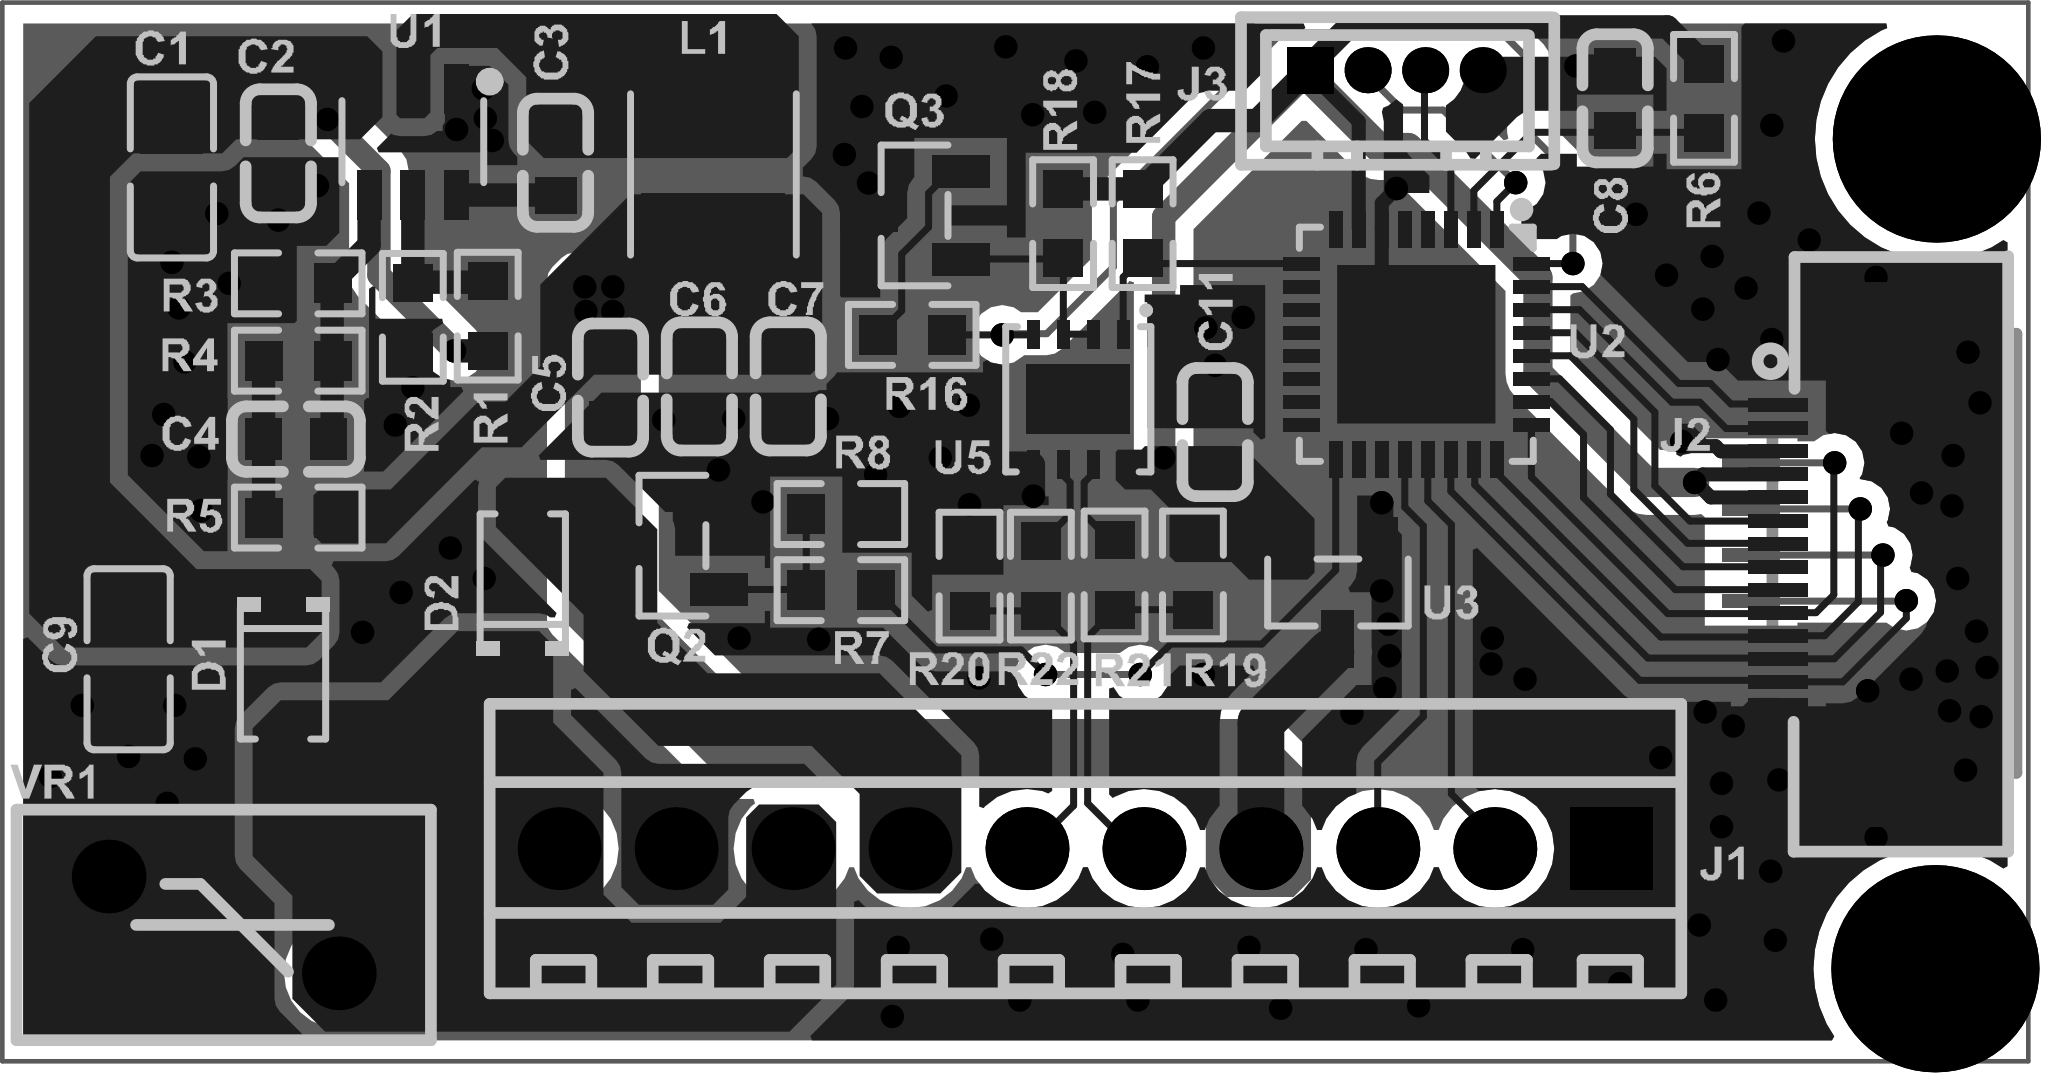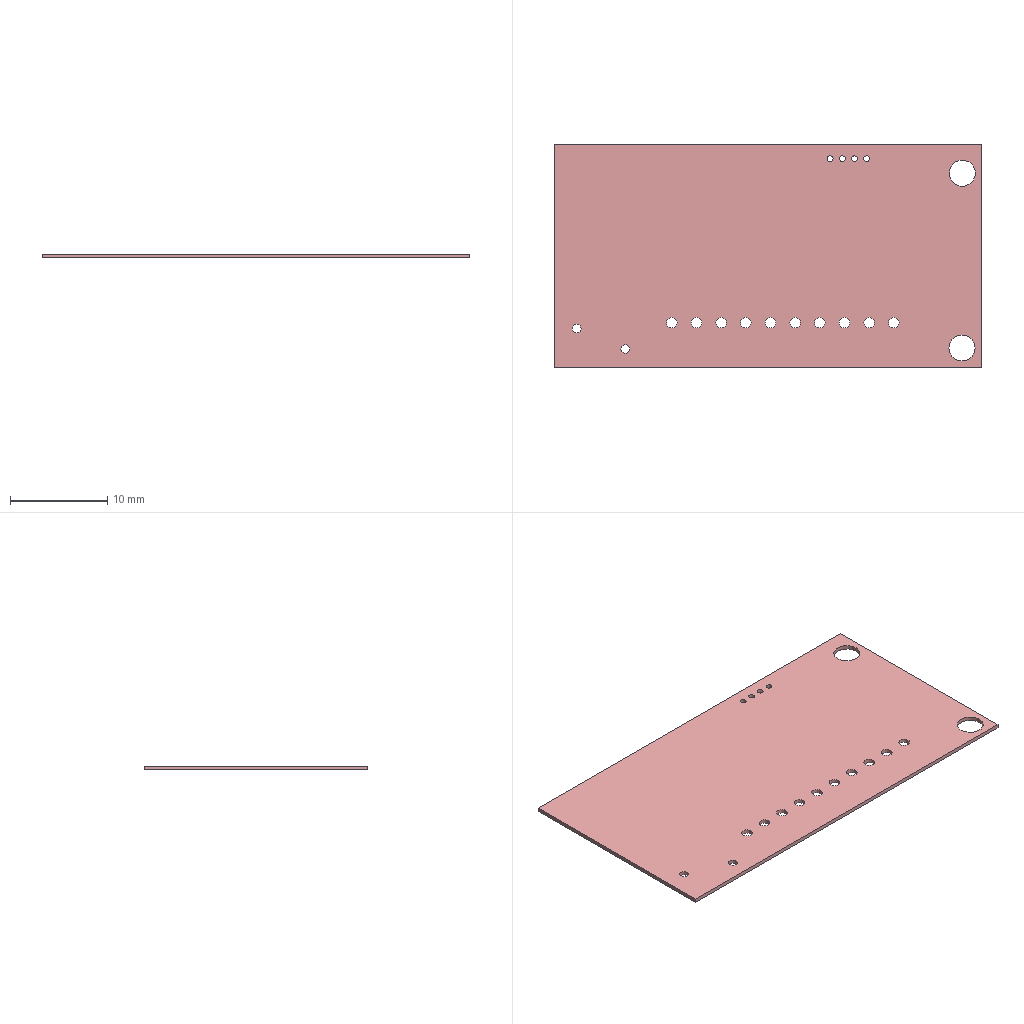Circuit board layout | Altium Designer | box 44 x 23 x 0.4 mm
Layer stack:
# Altium Designer layer stack of  (unit mm; dielectric type: 0 none, 1 core, 2 prepreg, 3 surface material)
index,name,kind,layer,copper_thickness_mm,dielectric_type,dielectric_thickness_mm,dielectric_material,dielectric_constant
0,Top Paste,other,,,,,,
1,Top Overlay,other,,,,,,
2,Top Solder,dielectric,,,3,0.0102,Solder Resist,3.5
3,Top Layer,copper,Top Layer,0.0356,,,,
4,Dielectric1,dielectric,,,0,0.32,FR-4,4.8
5,Bottom Layer,copper,Bottom Layer,0.0356,,,,
6,Bottom Solder,dielectric,,,3,0.0102,Solder Resist,3.5
7,Bottom Overlay,other,,,,,,
8,Bottom Paste,other,,,,,,
# drill layer pairs: low layer,high layer
drill_pair,Top Layer,Bottom Layer
Part placement:
Designator,Comment,Layer,Footprint,Center-X(mm),Center-Y(mm),Rotation
VR1,RES-TH_L9.0-W5.0-P5.00-D0.8-S2.10,TopLayer,RES-TH_L9.0-W5.0-P5.00-D0.8-S2.10,71.077,72.978,0
U5,SIT3088ETK,TopLayer,DFN-8_L3.0-W3.0-P0.65-BL-EP,89.637,84.379,180
U3,H7233-1,TopLayer,SOT-23-3_L2.9-W1.3-P1.90-LS2.4-BR,95.275,80.188,90
U2,QFN-32_L5.0-W5.0-P0.50-TL-EP3.1,TopLayer,QFN-32_L5.0-W5.0-P0.50-TL-EP3.1,96.977,85.573,270
U1,TPS54202DDCR,TopLayer,SOT-23-6_L2.9-W1.6-P0.95-LS2.8-BL,75.184,89.967,180
R22,,TopLayer,R0603,88.824,80.543,90
R21,,TopLayer,R0603,90.424,80.569,90
R20,,TopLayer,R0603,87.274,80.543,90
R19,,TopLayer,R0603,92.126,80.569,90
R18,,TopLayer,R0603,89.306,88.189,270
R17,,TopLayer,R0603,91.034,88.189,270
R16,,TopLayer,R0603,86.03,85.776,360
R8,,TopLayer,R0603,84.48,81.89,360
R7,,TopLayer,R0603,84.48,80.239,180
R6,,TopLayer,R0603,103.226,90.907,270
R5,,TopLayer,R0603,72.695,81.813,180
R4,,TopLayer,R0603,72.695,85.217,180
R3,,TopLayer,R0603,72.695,86.893,180
R2,,TopLayer,R0603,75.184,86.157,270
R1,,TopLayer,R0603,76.81,86.182,90
Q3,SS8050,TopLayer,SOT-23-3_L2.9-W1.3-P1.90-LS2.4-BR,86.081,88.367,360
Q2,AO3400,TopLayer,SOT-23-3_L2.9-W1.3-P1.90-LS2.4-BL-2,80.823,81.204,90
L1,15uH,TopLayer,IND-SMD_L3.5-W3.0,81.712,89.256,90
J4,AFA01-S05FCA-00,TopLayer,FPC-SMD_AFA01-S05FCA-00,105.512,81.001,270
J2,AFC07-S14FCA-00,TopLayer,FPC-SMD_14P-P0.50_AFC07-S14FCA-00,105.966,81.005,90
J1,CONN-TH_DB125-2.54-10P-GN,TopLayer,CONN-TH_DB125-2.54-10P-GN,89.792,74.633,180
D2,1N4148,TopLayer,SOD-123_L2.7-W1.7-LS3.8-RD,77.572,80.467,90
D1,1N4148,TopLayer,SOD-123_L2.7-W1.7-LS3.8-RD,72.365,78.435,270
C11,0.1uf 50V,TopLayer,C0603,92.608,83.668,270
C8,0.1uf 50V,TopLayer,C0603,101.295,90.907,270
C7,22uf 10V,TopLayer,C0603,83.337,84.658,270
C6,22uf 10V,TopLayer,C0603,81.407,84.658,270
C5,22uf 10V,TopLayer,C0603,79.477,84.633,270
C4,75pf,TopLayer,C0603,72.644,83.515,360
C3,0.1uf 50V,TopLayer,C0603,78.283,89.51,270
C2,0.1uf 50V,TopLayer,C0603,72.263,89.713,90
C1,10uF 35V,TopLayer,C0805,69.952,89.408,270
J3,HC-1.25-4A,TopLayer,CONN-TH_4P-P1.25_HCTL_HC-1.25-4A,96.545,91.516,360
C9,10uF 35V,TopLayer,C0805,69.012,78.74,270
Pad and via stacks:
# Altium Designer via and pad stacks of  (unit mm). Each distinct definition once, with the count of objects using it.
# via: kind,start_layer,end_layer,hole_mm,diameter_mm,mode(0 simple;1 top-mid-bottom;2 full stack),diameter_per_layer,count,example_net
# pad: kind,layer,hole_mm,hole_type(0 round;1 square;2 slot),plating,top_size,top_shape(1 round;2 rect;3 octagon;9 rounded rect),mid_size,bottom_size,mode,footprint,size_per_layer,count,example
pad,Multi-Layer,2.7,0,plated,4.5x4.5,1,4.5x4.5,4.5x4.5,0,,,2,0
pad,Multi-Layer,0.6,0,plated,1x1,2,1x1,1x1,0,CONN-TH_4P-P1.25_HCTL_HC-1.25-4A,,1,J3.1
pad,Multi-Layer,0.6,0,plated,1x1,1,1x1,1x1,0,CONN-TH_4P-P1.25_HCTL_HC-1.25-4A,,3,J3.2
pad,Multi-Layer,1.1,0,plated,1.8x1.8,1,1.8x1.8,1.8x1.8,0,CONN-TH_DB125-2.54-10P-GN,,9,J1.10
pad,Multi-Layer,1.1,0,plated,1.8x1.8,2,1.8x1.8,1.8x1.8,0,CONN-TH_DB125-2.54-10P-GN,,1,J1.1
pad,Multi-Layer,0.9,0,plated,1.6x1.6,1,1.6x1.6,1.6x1.6,0,RES-TH_L9.0-W5.0-P5.00-D0.8-S2.10,,2,VR1.1
pad,Top Layer,0,0,plated,0.3x1.3,2,0.3x1.3,0.3x1.3,0,FPC-SMD_14P-P0.50_AFC07-S14FCA-00,,14,J2.1
pad,Top Layer,0,0,plated,2x3,2,2x3,2x3,0,FPC-SMD_14P-P0.50_AFC07-S14FCA-00,,2,J2.16
pad,Top Layer,0,0,plated,1.25x0.7,2,1.25x0.7,1.25x0.7,0,SOT-23-3_L2.9-W1.3-P1.90-LS2.4-BR,,6,U3.1
pad,Top Layer,0,0,plated,0.8065x0.864,2,0.8065x0.864,0.8065x0.864,0,R0603,,30,R22.2
pad,Top Layer,0,0,plated,0.91x0.84,2,0.91x0.84,0.91x0.84,0,SOD-123_L2.7-W1.7-LS3.8-RD,,4,D2.1
pad,Top Layer,0,0,plated,0.8x0.9,2,0.8x0.9,0.8x0.9,0,C0603,,16,C11.2
pad,Top Layer,0,0,plated,1.41x1.35,2,1.41x1.35,1.41x1.35,0,C0805,,4,C1.2
pad,Top Layer,0,0,plated,1.8x3.12,2,1.8x3.12,1.8x3.12,0,IND-SMD_L3.5-W3.0,,2,L1.1
pad,Top Layer,0,0,plated,1.25x0.7,2,1.25x0.7,1.25x0.7,0,SOT-23-3_L2.9-W1.3-P1.90-LS2.4-BL-2,,3,Q2.3
pad,Top Layer,0,0,plated,0.532x1.072,2,0.532x1.072,0.532x1.072,0,SOT-23-6_L2.9-W1.6-P0.95-LS2.8-BL,,6,U1.1
pad,Top Layer,0,0,plated,3.2x3.2,2,3.2x3.2,3.2x3.2,0,QFN-32_L5.0-W5.0-P0.50-TL-EP3.1,,1,U2.33
pad,Top Layer,0,0,plated,0.3x0.8,2,0.3x0.8,0.3x0.8,0,QFN-32_L5.0-W5.0-P0.50-TL-EP3.1,,32,U2.32
pad,Top Layer,0,0,plated,0.28x0.625,2,0.28x0.625,0.28x0.625,0,DFN-8_L3.0-W3.0-P0.65-BL-EP,,8,U5.1
pad,Top Layer,0,0,plated,2.25x1.5,2,2.25x1.5,2.25x1.5,0,DFN-8_L3.0-W3.0-P0.65-BL-EP,,1,U5.9
pad,Bottom Layer,0,0,plated,1.25x0.3,2,1.25x0.3,1.25x0.3,0,FPC-SMD_AFA01-S05FCA-00,,5,J4.1
pad,Bottom Layer,0,0,plated,2x2.5,2,2x2.5,2x2.5,0,FPC-SMD_AFA01-S05FCA-00,,2,J4.6
via,Top Layer,Bottom Layer,0.3048,0.508,0,,145,3.3V
Copper pours:
name,layer,net,type(0 solid;1 hatched;2 none)
Bottom Layer-No Net,Top Layer,PWMO,0
Bottom Layer-No Net,Top Layer,VCC,0
Bottom Layer-No Net,Top Layer,3.3V,0
Bottom Layer-No Net,Top Layer,VIN,0
Bottom Layer-No Net,Top Layer,SW,0
Bottom Layer-No Net,Top Layer,+5V,0
Bottom Layer-No Net,Top Layer,GND,0
Bottom Layer-No Net,Bottom Layer,+5V,0
Bottom Layer-No Net,Bottom Layer,GND,0
Design rules, without the lines most boards share:
# Altium Designer design rules of  (exported by Altium Designer, unit mm)
# columns: name | kind | enabled | priority | scope1 | scope2 | descriptor | typed fields (field=value)
Clearance | 0 | enabled | 2 | All | All | Clearance Constraint (Gap=6mil) (All),(All) | gap=0.1524
PlaneConnect | 6 | enabled | 1 | All | All | Power Plane Connect Rule(Direct Connect )(Expansion=20mil) (Conductor Width=10mil) (Air Gap=10mil) (Entries=4) (All) | relief_conductor_width=0.254 relief_entries=4 relief_expansion=0.508
PlaneClearance | 12 | enabled | 1 | All | All | Power Plane Clearance (Clearance =6mil) (All) | clearance=0.1524
PolygonConnect | 20 | enabled | 1 | All | All | Polygon Connect Rule(Direct Connect )(Conductor Width=10mil) (Relief Angle=90 Angle) (Entries=4) (Air Gap Width=10mil) (All),(All) | connect_style(0=relief,1=direct,2=none)=1 relief_conductor_width=0.254 relief_entries=4
Width | 2 | enabled | 1 | All | All | Width Constraint (Min=6mil) (Max=40mil) (Preferred=6mil) (All) |
RoutingVias | 11 | enabled | 1 | All | All | Routing Via (MinHoleWidth=12mil) (MaxHoleWidth=12mil) (PreferredHoleWidth=12mil) (MinWidth=20mil) (MaxWidth=20mil) (PreferedWidth=20mil) (All) | via_min_hole=0.3048 via_max_hole=0.3048 via_preferred_diameter=0.508 via_preferred_hole=0.3048
PasteMaskExpansion | 14 | enabled | 1 | All | All | Paste Mask Expansion (Expansion =0mil) (All) | expansion=0
SolderMaskExpansion | 13 | enabled | 1 | All | All | Solder Mask Expansion (Expansion =4mil) (All) | expansion=0.1016
HoleSize | 42 | enabled | 1 | All | All | Hole Size Constraint (Min=1mil) (Max=500mil) (All) |
DiffPairsRouting | 51 | enabled | 1 | All | All | Differential Pairs Uncoupled Length using the Gap Constraints (Min=10mil) (Max=10mil) (Prefered=10mil)  and Width Constraints (Min=15mil) (Max=15mil) (Prefered=15mil) (All) |
HoleToHoleClearance | 52 | enabled | 1 | All | All | Hole To Hole Clearance (Gap=0mil) (All),(All) | gap=0
MinimumSolderMaskSliver | 53 | enabled | 1 | All | All | Minimum Solder Mask Sliver (Gap=0mil) (All),(All) |
SilkscreenOverComponentPads | 54 | enabled | 1 | IsPad | All | Silk To Solder Mask (Clearance=0mil) (IsPad),(All) |
SilkToSilkClearance | 55 | enabled | 1 | All | All | Silk to Silk (Clearance=0mil) (All),(All) |
Clearance_1 | 0 | enabled | 1 | inpolygon | All | Clearance Constraint (Gap=6mil) (inpolygon),(All) | gap=0.1524
Classes set for this board:
# Altium Designer classes of  (member kind: 0 net, 1 component, 2 from-to, 3 pad, 4 layer, 5 differential pair, 6 design channel, 7 polygon, 8 structure, 9 xSignal)
# columns: class name | member kind | superclass | members
1_P1 | 1 | no | C1; C2; C3; C4; C5; C6; C7; C8; C11; D1; D2; J1; J2; J3; J4; L1; Q2; Q3; R1; R2; R3; R4; R5; R6; R7; R8; R16; R17; R18; R19; R20; R21; R22; U1; U2; U3; U5; VR1; C9;